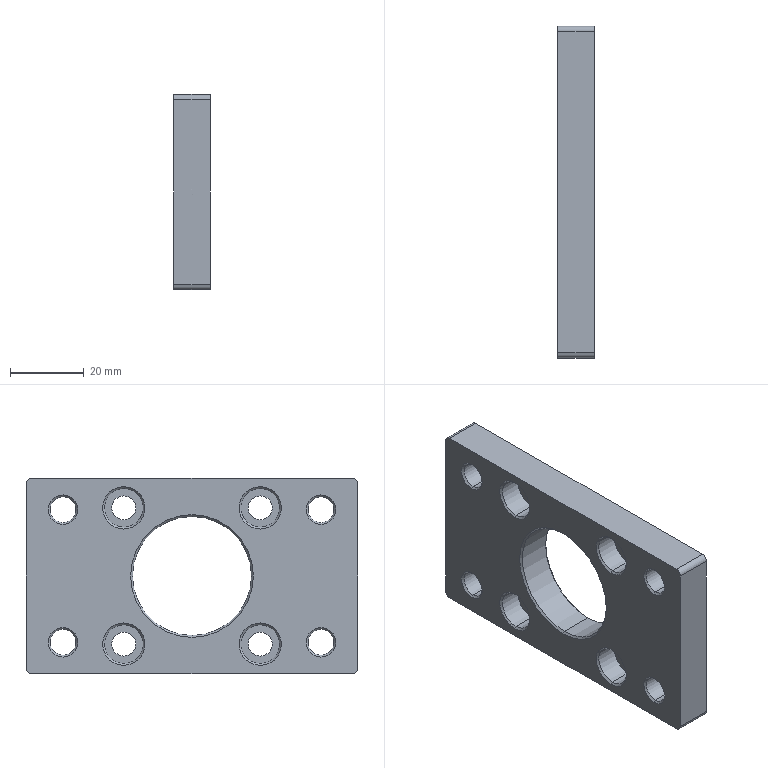Part | STEP file | 03-30SC气缸垫块 | 1 solid | 60 faces | box 10 x 90 x 53 mm | volume 35177 mm3 | cylinder 30 | cone 20 | plane 10 | commonest cylinder face diameters 6.5 x8 7 x8 10.5 x8 3 x4 32.3 x2